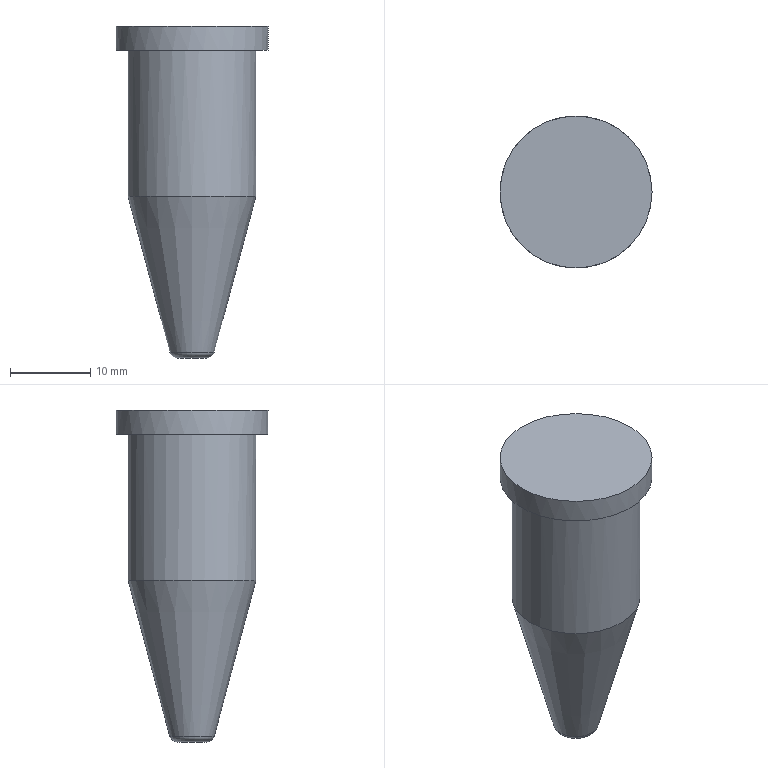Part | STEP file | lll_id2782_x_t | 1 solid | 7 faces | box 19 x 19 x 41.5 mm | volume 6462 mm3 | plane 3 | cylinder 2 | cone 1 | torus 1 | commonest cylinder face diameters 16 x1 19 x1
STEP:
#1=CARTESIAN_POINT('',(3564.,-1.821,-19.));
#2=VERTEX_POINT('',#1);
#3=CARTESIAN_POINT('',(3564.,0.,-19.));
#4=DIRECTION('',(0.,0.,-1.));
#5=DIRECTION('',(0.,-1.,0.));
#6=AXIS2_PLACEMENT_3D('',#3,#4,#5);
#7=CIRCLE('',#6,1.821);
#8=EDGE_CURVE('',#2,#2,#7,.T.);
#9=ORIENTED_EDGE('',*,*,#8,.T.);
#10=EDGE_LOOP('',(#9));
#11=FACE_OUTER_BOUND('',#10,.T.);
#12=CARTESIAN_POINT('',(3564.,0.,-19.));
#13=DIRECTION('',(0.,0.,1.));
#14=DIRECTION('',(0.,-1.,0.));
#15=AXIS2_PLACEMENT_3D('',#12,#13,#14);
#16=PLANE('',#15);
#17=ADVANCED_FACE('',(#11),#16,.F.);
#18=CARTESIAN_POINT('',(3573.5,0.,19.5));
#19=VERTEX_POINT('',#18);
#20=CARTESIAN_POINT('',(3564.,0.,19.5));
#21=DIRECTION('',(0.,0.,-1.));
#22=DIRECTION('',(1.,0.,0.));
#23=AXIS2_PLACEMENT_3D('',#20,#21,#22);
#24=CIRCLE('',#23,9.5);
#25=EDGE_CURVE('',#19,#19,#24,.T.);
#26=ORIENTED_EDGE('',*,*,#25,.T.);
#27=EDGE_LOOP('',(#26));
#28=FACE_BOUND('',#27,.T.);
#29=CARTESIAN_POINT('',(3572.,0.,19.5));
#30=VERTEX_POINT('',#29);
#31=CARTESIAN_POINT('',(3564.,0.,19.5));
#32=DIRECTION('',(0.,0.,1.));
#33=DIRECTION('',(1.,0.,0.));
#34=AXIS2_PLACEMENT_3D('',#31,#32,#33);
#35=CIRCLE('',#34,8.);
#36=EDGE_CURVE('',#30,#30,#35,.T.);
#37=ORIENTED_EDGE('',*,*,#36,.T.);
#38=EDGE_LOOP('',(#37));
#39=FACE_BOUND('',#38,.T.);
#40=CARTESIAN_POINT('',(3564.,0.,19.5));
#41=DIRECTION('',(0.,0.,-1.));
#42=DIRECTION('',(0.,1.,0.));
#43=AXIS2_PLACEMENT_3D('',#40,#41,#42);
#44=PLANE('',#43);
#45=ADVANCED_FACE('',(#28,#39),#44,.T.);
#46=CARTESIAN_POINT('',(3554.5,0.,22.5));
#47=VERTEX_POINT('',#46);
#48=CARTESIAN_POINT('',(3564.,0.,22.5));
#49=DIRECTION('',(0.,0.,1.));
#50=DIRECTION('',(-1.,0.,0.));
#51=AXIS2_PLACEMENT_3D('',#48,#49,#50);
#52=CIRCLE('',#51,9.5);
#53=EDGE_CURVE('',#47,#47,#52,.T.);
#54=ORIENTED_EDGE('',*,*,#53,.F.);
#55=EDGE_LOOP('',(#54));
#56=FACE_BOUND('',#55,.T.);
#57=ORIENTED_EDGE('',*,*,#25,.F.);
#58=EDGE_LOOP('',(#57));
#59=FACE_BOUND('',#58,.T.);
#60=CARTESIAN_POINT('',(3564.,0.,19.5));
#61=DIRECTION('',(0.,0.,-1.));
#62=DIRECTION('',(0.,1.,0.));
#63=AXIS2_PLACEMENT_3D('',#60,#61,#62);
#64=CYLINDRICAL_SURFACE('',#63,9.5);
#65=ADVANCED_FACE('',(#56,#59),#64,.T.);
#66=ORIENTED_EDGE('',*,*,#53,.T.);
#67=EDGE_LOOP('',(#66));
#68=FACE_OUTER_BOUND('',#67,.T.);
#69=CARTESIAN_POINT('',(3564.,0.,22.5));
#70=DIRECTION('',(0.,0.,1.));
#71=DIRECTION('',(0.,-1.,0.));
#72=AXIS2_PLACEMENT_3D('',#69,#70,#71);
#73=PLANE('',#72);
#74=ADVANCED_FACE('',(#68),#73,.T.);
#75=CARTESIAN_POINT('',(3556.,0.,1.196));
#76=VERTEX_POINT('',#75);
#77=CARTESIAN_POINT('',(3564.,0.,1.196));
#78=DIRECTION('',(0.,0.,1.));
#79=DIRECTION('',(-1.,0.,0.));
#80=AXIS2_PLACEMENT_3D('',#77,#78,#79);
#81=CIRCLE('',#80,8.);
#82=EDGE_CURVE('',#76,#76,#81,.T.);
#83=ORIENTED_EDGE('',*,*,#82,.T.);
#84=EDGE_LOOP('',(#83));
#85=FACE_BOUND('',#84,.T.);
#86=ORIENTED_EDGE('',*,*,#36,.F.);
#87=EDGE_LOOP('',(#86));
#88=FACE_BOUND('',#87,.T.);
#89=CARTESIAN_POINT('',(3564.,0.,20.5));
#90=DIRECTION('',(0.,0.,-1.));
#91=DIRECTION('',(0.,1.,0.));
#92=AXIS2_PLACEMENT_3D('',#89,#90,#91);
#93=CYLINDRICAL_SURFACE('',#92,8.);
#94=ADVANCED_FACE('',(#85,#88),#93,.T.);
#95=CARTESIAN_POINT('',(3564.,-2.787,-18.259));
#96=VERTEX_POINT('',#95);
#97=CARTESIAN_POINT('',(3564.,0.,-18.259));
#98=DIRECTION('',(0.,0.,1.));
#99=DIRECTION('',(0.,-1.,0.));
#100=AXIS2_PLACEMENT_3D('',#97,#98,#99);
#101=CIRCLE('',#100,2.787);
#102=EDGE_CURVE('',#96,#96,#101,.T.);
#103=ORIENTED_EDGE('',*,*,#102,.T.);
#104=EDGE_LOOP('',(#103));
#105=FACE_BOUND('',#104,.T.);
#106=ORIENTED_EDGE('',*,*,#82,.F.);
#107=EDGE_LOOP('',(#106));
#108=FACE_BOUND('',#107,.T.);
#109=CARTESIAN_POINT('',(3564.,0.,-19.));
#110=DIRECTION('',(0.,0.,1.));
#111=DIRECTION('',(0.,-1.,0.));
#112=AXIS2_PLACEMENT_3D('',#109,#110,#111);
#113=CONICAL_SURFACE('',#112,2.588,15.);
#114=ADVANCED_FACE('',(#105,#108),#113,.T.);
#115=ORIENTED_EDGE('',*,*,#102,.F.);
#116=EDGE_LOOP('',(#115));
#117=FACE_BOUND('',#116,.T.);
#118=ORIENTED_EDGE('',*,*,#8,.F.);
#119=EDGE_LOOP('',(#118));
#120=FACE_BOUND('',#119,.T.);
#121=CARTESIAN_POINT('',(3564.,0.,-18.));
#122=DIRECTION('',(0.,0.,1.));
#123=DIRECTION('',(0.,-1.,0.));
#124=AXIS2_PLACEMENT_3D('',#121,#122,#123);
#125=TOROIDAL_SURFACE('',#124,1.821,1.);
#126=ADVANCED_FACE('',(#117,#120),#125,.T.);
#127=CLOSED_SHELL('',(#17,#45,#65,#74,#94,#114,#126));
#128=MANIFOLD_SOLID_BREP('',#127);
#129=(LENGTH_UNIT()NAMED_UNIT(*)SI_UNIT(.MILLI.,.METRE.));
#130=UNCERTAINTY_MEASURE_WITH_UNIT(LENGTH_MEASURE(0.00002),#129,'','');
#131=(NAMED_UNIT(*)PLANE_ANGLE_UNIT()SI_UNIT($,.RADIAN.));
#132=PLANE_ANGLE_MEASURE_WITH_UNIT(PLANE_ANGLE_MEASURE(0.01745),#131);
#133=DIMENSIONAL_EXPONENTS(0.,0.,0.,0.,0.,0.,0.);
#134=(CONVERSION_BASED_UNIT('DEGREE',#132)NAMED_UNIT(#133)PLANE_ANGLE_UNIT());
#135=(NAMED_UNIT(*)SI_UNIT($,.STERADIAN.)SOLID_ANGLE_UNIT());
#136=(GEOMETRIC_REPRESENTATION_CONTEXT(3)GLOBAL_UNCERTAINTY_ASSIGNED_CONTEXT((#130))GLOBAL_UNIT_ASSIGNED_CONTEXT((#129,#134,#135))REPRESENTATION_CONTEXT('',''));
#137=ADVANCED_BREP_SHAPE_REPRESENTATION('',(#128),#136);